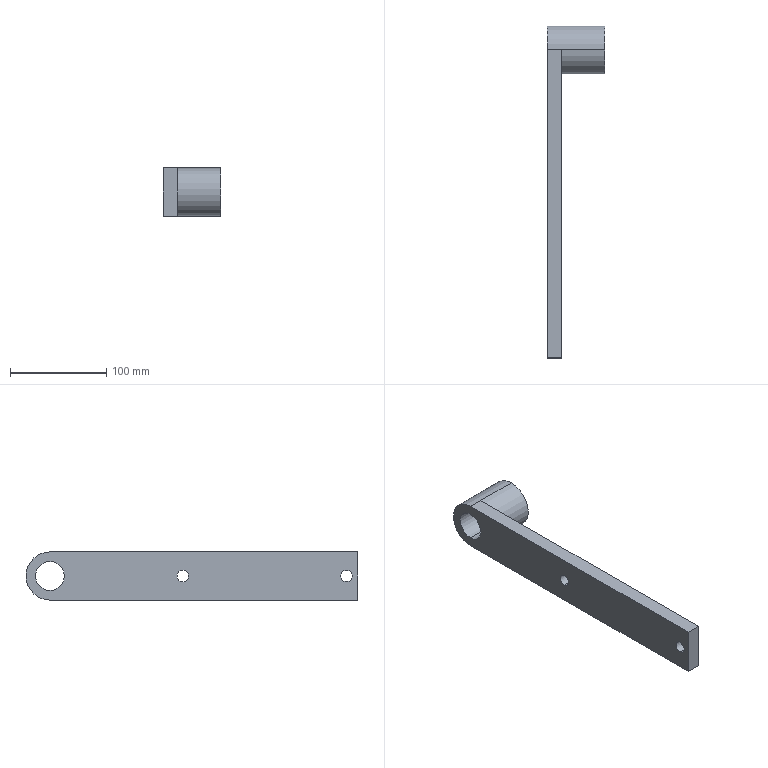Part | SolidWorks | features ICE 2, Extrusion 1, HoleWzd 1 | 1 solid | 14 faces | box 60 x 345 x 50 mm | volume 297279 mm3 | cylinder 8 | plane 6 | commonest cylinder face diameters 12 x4 30 x2 50 x2
STEP:
#1=CARTESIAN_POINT('',(7.5,22.,6.));
#2=VERTEX_POINT('',#1);
#3=CARTESIAN_POINT('',(7.5,22.,-6.));
#4=VERTEX_POINT('',#3);
#5=CARTESIAN_POINT('',(7.5,22.,0.));
#6=DIRECTION('',(1.,0.,0.));
#7=DIRECTION('',(0.,0.,-1.));
#8=AXIS2_PLACEMENT_3D('',#5,#6,#7);
#9=CIRCLE('',#8,6.);
#10=EDGE_CURVE('',#2,#4,#9,.T.);
#11=ORIENTED_EDGE('',*,*,#10,.T.);
#12=CARTESIAN_POINT('',(-7.5,22.,-6.));
#13=VERTEX_POINT('',#12);
#14=CARTESIAN_POINT('',(-7.5,22.,-6.));
#15=DIRECTION('',(-1.,0.,0.));
#16=VECTOR('',#15,1000.);
#17=LINE('',#14,#16);
#18=EDGE_CURVE('',#4,#13,#17,.T.);
#19=ORIENTED_EDGE('',*,*,#18,.T.);
#20=CARTESIAN_POINT('',(-7.5,22.,6.));
#21=VERTEX_POINT('',#20);
#22=CARTESIAN_POINT('',(-7.5,22.,0.));
#23=DIRECTION('',(-1.,0.,0.));
#24=DIRECTION('',(0.,0.,1.));
#25=AXIS2_PLACEMENT_3D('',#22,#23,#24);
#26=CIRCLE('',#25,6.);
#27=EDGE_CURVE('',#13,#21,#26,.T.);
#28=ORIENTED_EDGE('',*,*,#27,.T.);
#29=CARTESIAN_POINT('',(-7.5,22.,6.));
#30=DIRECTION('',(-1.,0.,0.));
#31=VECTOR('',#30,1000.);
#32=LINE('',#29,#31);
#33=EDGE_CURVE('',#2,#21,#32,.T.);
#34=ORIENTED_EDGE('',*,*,#33,.F.);
#35=EDGE_LOOP('',(#11,#19,#28,#34));
#36=FACE_OUTER_BOUND('',#35,.T.);
#37=CARTESIAN_POINT('',(-7.5,22.,0.));
#38=DIRECTION('',(-1.,0.,0.));
#39=DIRECTION('',(0.,0.,1.));
#40=AXIS2_PLACEMENT_3D('',#37,#38,#39);
#41=CYLINDRICAL_SURFACE('',#40,6.);
#42=ADVANCED_FACE('',(#36),#41,.F.);
#43=CARTESIAN_POINT('',(7.5,-148.,6.));
#44=VERTEX_POINT('',#43);
#45=CARTESIAN_POINT('',(7.5,-148.,-6.));
#46=VERTEX_POINT('',#45);
#47=CARTESIAN_POINT('',(7.5,-148.,0.));
#48=DIRECTION('',(1.,0.,0.));
#49=DIRECTION('',(0.,0.,-1.));
#50=AXIS2_PLACEMENT_3D('',#47,#48,#49);
#51=CIRCLE('',#50,6.);
#52=EDGE_CURVE('',#44,#46,#51,.T.);
#53=ORIENTED_EDGE('',*,*,#52,.T.);
#54=CARTESIAN_POINT('',(-7.5,-148.,-6.));
#55=VERTEX_POINT('',#54);
#56=CARTESIAN_POINT('',(-7.5,-148.,-6.));
#57=DIRECTION('',(-1.,0.,0.));
#58=VECTOR('',#57,1000.);
#59=LINE('',#56,#58);
#60=EDGE_CURVE('',#46,#55,#59,.T.);
#61=ORIENTED_EDGE('',*,*,#60,.T.);
#62=CARTESIAN_POINT('',(-7.5,-148.,6.));
#63=VERTEX_POINT('',#62);
#64=CARTESIAN_POINT('',(-7.5,-148.,0.));
#65=DIRECTION('',(-1.,0.,0.));
#66=DIRECTION('',(0.,0.,1.));
#67=AXIS2_PLACEMENT_3D('',#64,#65,#66);
#68=CIRCLE('',#67,6.);
#69=EDGE_CURVE('',#55,#63,#68,.T.);
#70=ORIENTED_EDGE('',*,*,#69,.T.);
#71=CARTESIAN_POINT('',(-7.5,-148.,6.));
#72=DIRECTION('',(-1.,0.,0.));
#73=VECTOR('',#72,1000.);
#74=LINE('',#71,#73);
#75=EDGE_CURVE('',#44,#63,#74,.T.);
#76=ORIENTED_EDGE('',*,*,#75,.F.);
#77=EDGE_LOOP('',(#53,#61,#70,#76));
#78=FACE_OUTER_BOUND('',#77,.T.);
#79=CARTESIAN_POINT('',(-7.5,-148.,0.));
#80=DIRECTION('',(-1.,0.,0.));
#81=DIRECTION('',(0.,0.,1.));
#82=AXIS2_PLACEMENT_3D('',#79,#80,#81);
#83=CYLINDRICAL_SURFACE('',#82,6.);
#84=ADVANCED_FACE('',(#78),#83,.F.);
#85=CARTESIAN_POINT('',(-7.5,160.,15.));
#86=VERTEX_POINT('',#85);
#87=CARTESIAN_POINT('',(-7.5,160.,-15.));
#88=VERTEX_POINT('',#87);
#89=CARTESIAN_POINT('',(-7.5,160.,0.));
#90=DIRECTION('',(1.,0.,0.));
#91=DIRECTION('',(0.,0.,-1.));
#92=AXIS2_PLACEMENT_3D('',#89,#90,#91);
#93=CIRCLE('',#92,15.);
#94=EDGE_CURVE('',#86,#88,#93,.T.);
#95=ORIENTED_EDGE('',*,*,#94,.F.);
#96=CARTESIAN_POINT('',(52.5,160.,15.));
#97=VERTEX_POINT('',#96);
#98=CARTESIAN_POINT('',(-7.5,160.,15.));
#99=DIRECTION('',(1.,0.,0.));
#100=VECTOR('',#99,1000.);
#101=LINE('',#98,#100);
#102=EDGE_CURVE('',#86,#97,#101,.T.);
#103=ORIENTED_EDGE('',*,*,#102,.T.);
#104=CARTESIAN_POINT('',(52.5,160.,-15.));
#105=VERTEX_POINT('',#104);
#106=CARTESIAN_POINT('',(52.5,160.,0.));
#107=DIRECTION('',(1.,0.,0.));
#108=DIRECTION('',(0.,0.,-1.));
#109=AXIS2_PLACEMENT_3D('',#106,#107,#108);
#110=CIRCLE('',#109,15.);
#111=EDGE_CURVE('',#97,#105,#110,.T.);
#112=ORIENTED_EDGE('',*,*,#111,.T.);
#113=CARTESIAN_POINT('',(-7.5,160.,-15.));
#114=DIRECTION('',(1.,0.,0.));
#115=VECTOR('',#114,1000.);
#116=LINE('',#113,#115);
#117=EDGE_CURVE('',#88,#105,#116,.T.);
#118=ORIENTED_EDGE('',*,*,#117,.F.);
#119=EDGE_LOOP('',(#95,#103,#112,#118));
#120=FACE_OUTER_BOUND('',#119,.T.);
#121=CARTESIAN_POINT('',(-7.5,160.,0.));
#122=DIRECTION('',(1.,0.,0.));
#123=DIRECTION('',(0.,0.,-1.));
#124=AXIS2_PLACEMENT_3D('',#121,#122,#123);
#125=CYLINDRICAL_SURFACE('',#124,15.);
#126=ADVANCED_FACE('',(#120),#125,.F.);
#127=CARTESIAN_POINT('',(7.5,160.,25.));
#128=VERTEX_POINT('',#127);
#129=CARTESIAN_POINT('',(-7.5,160.,25.));
#130=VERTEX_POINT('',#129);
#131=CARTESIAN_POINT('',(7.5,160.,25.));
#132=DIRECTION('',(-1.,0.,0.));
#133=VECTOR('',#132,1000.);
#134=LINE('',#131,#133);
#135=EDGE_CURVE('',#128,#130,#134,.T.);
#136=ORIENTED_EDGE('',*,*,#135,.F.);
#137=CARTESIAN_POINT('',(52.5,160.,25.));
#138=VERTEX_POINT('',#137);
#139=CARTESIAN_POINT('',(-7.5,160.,25.));
#140=DIRECTION('',(1.,0.,0.));
#141=VECTOR('',#140,1000.);
#142=LINE('',#139,#141);
#143=EDGE_CURVE('',#128,#138,#142,.T.);
#144=ORIENTED_EDGE('',*,*,#143,.T.);
#145=CARTESIAN_POINT('',(52.5,160.,-25.));
#146=VERTEX_POINT('',#145);
#147=CARTESIAN_POINT('',(52.5,160.,0.));
#148=DIRECTION('',(1.,0.,0.));
#149=DIRECTION('',(0.,0.,-1.));
#150=AXIS2_PLACEMENT_3D('',#147,#148,#149);
#151=CIRCLE('',#150,25.);
#152=EDGE_CURVE('',#146,#138,#151,.T.);
#153=ORIENTED_EDGE('',*,*,#152,.F.);
#154=CARTESIAN_POINT('',(7.5,160.,-25.));
#155=VERTEX_POINT('',#154);
#156=CARTESIAN_POINT('',(-7.5,160.,-25.));
#157=DIRECTION('',(1.,0.,0.));
#158=VECTOR('',#157,1000.);
#159=LINE('',#156,#158);
#160=EDGE_CURVE('',#155,#146,#159,.T.);
#161=ORIENTED_EDGE('',*,*,#160,.F.);
#162=CARTESIAN_POINT('',(-7.5,160.,-25.));
#163=VERTEX_POINT('',#162);
#164=CARTESIAN_POINT('',(7.5,160.,-25.));
#165=DIRECTION('',(-1.,0.,0.));
#166=VECTOR('',#165,1000.);
#167=LINE('',#164,#166);
#168=EDGE_CURVE('',#155,#163,#167,.T.);
#169=ORIENTED_EDGE('',*,*,#168,.T.);
#170=CARTESIAN_POINT('',(-7.5,160.,0.));
#171=DIRECTION('',(1.,0.,0.));
#172=DIRECTION('',(0.,0.,-1.));
#173=AXIS2_PLACEMENT_3D('',#170,#171,#172);
#174=CIRCLE('',#173,25.);
#175=EDGE_CURVE('',#163,#130,#174,.T.);
#176=ORIENTED_EDGE('',*,*,#175,.T.);
#177=EDGE_LOOP('',(#136,#144,#153,#161,#169,#176));
#178=FACE_OUTER_BOUND('',#177,.T.);
#179=CARTESIAN_POINT('',(-7.5,160.,0.));
#180=DIRECTION('',(1.,0.,0.));
#181=DIRECTION('',(0.,0.,-1.));
#182=AXIS2_PLACEMENT_3D('',#179,#180,#181);
#183=CYLINDRICAL_SURFACE('',#182,25.);
#184=ADVANCED_FACE('',(#178),#183,.T.);
#185=CARTESIAN_POINT('',(-7.5,-160.,-25.));
#186=VERTEX_POINT('',#185);
#187=CARTESIAN_POINT('',(-7.5,160.,-25.));
#188=DIRECTION('',(0.,1.,0.));
#189=VECTOR('',#188,1000.);
#190=LINE('',#187,#189);
#191=EDGE_CURVE('',#186,#163,#190,.T.);
#192=ORIENTED_EDGE('',*,*,#191,.T.);
#193=ORIENTED_EDGE('',*,*,#168,.F.);
#194=CARTESIAN_POINT('',(7.5,-160.,-25.));
#195=VERTEX_POINT('',#194);
#196=CARTESIAN_POINT('',(7.5,160.,-25.));
#197=DIRECTION('',(0.,1.,0.));
#198=VECTOR('',#197,1000.);
#199=LINE('',#196,#198);
#200=EDGE_CURVE('',#195,#155,#199,.T.);
#201=ORIENTED_EDGE('',*,*,#200,.F.);
#202=CARTESIAN_POINT('',(7.5,-160.,-25.));
#203=DIRECTION('',(-1.,0.,0.));
#204=VECTOR('',#203,1000.);
#205=LINE('',#202,#204);
#206=EDGE_CURVE('',#195,#186,#205,.T.);
#207=ORIENTED_EDGE('',*,*,#206,.T.);
#208=EDGE_LOOP('',(#192,#193,#201,#207));
#209=FACE_OUTER_BOUND('',#208,.T.);
#210=CARTESIAN_POINT('',(7.5,160.,-25.));
#211=DIRECTION('',(0.,0.,1.));
#212=DIRECTION('',(0.,-1.,0.));
#213=AXIS2_PLACEMENT_3D('',#210,#211,#212);
#214=PLANE('',#213);
#215=ADVANCED_FACE('',(#209),#214,.F.);
#216=CARTESIAN_POINT('',(-7.5,-160.,25.));
#217=VERTEX_POINT('',#216);
#218=CARTESIAN_POINT('',(-7.5,160.,25.));
#219=DIRECTION('',(0.,-1.,0.));
#220=VECTOR('',#219,1000.);
#221=LINE('',#218,#220);
#222=EDGE_CURVE('',#130,#217,#221,.T.);
#223=ORIENTED_EDGE('',*,*,#222,.T.);
#224=CARTESIAN_POINT('',(7.5,-160.,25.));
#225=VERTEX_POINT('',#224);
#226=CARTESIAN_POINT('',(7.5,-160.,25.));
#227=DIRECTION('',(-1.,0.,0.));
#228=VECTOR('',#227,1000.);
#229=LINE('',#226,#228);
#230=EDGE_CURVE('',#225,#217,#229,.T.);
#231=ORIENTED_EDGE('',*,*,#230,.F.);
#232=CARTESIAN_POINT('',(7.5,160.,25.));
#233=DIRECTION('',(0.,-1.,0.));
#234=VECTOR('',#233,1000.);
#235=LINE('',#232,#234);
#236=EDGE_CURVE('',#128,#225,#235,.T.);
#237=ORIENTED_EDGE('',*,*,#236,.F.);
#238=ORIENTED_EDGE('',*,*,#135,.T.);
#239=EDGE_LOOP('',(#223,#231,#237,#238));
#240=FACE_OUTER_BOUND('',#239,.T.);
#241=CARTESIAN_POINT('',(7.5,160.,25.));
#242=DIRECTION('',(0.,0.,-1.));
#243=DIRECTION('',(0.,1.,0.));
#244=AXIS2_PLACEMENT_3D('',#241,#242,#243);
#245=PLANE('',#244);
#246=ADVANCED_FACE('',(#240),#245,.F.);
#247=CARTESIAN_POINT('',(-7.5,-160.,25.));
#248=DIRECTION('',(0.,0.,-1.));
#249=VECTOR('',#248,1000.);
#250=LINE('',#247,#249);
#251=EDGE_CURVE('',#217,#186,#250,.T.);
#252=ORIENTED_EDGE('',*,*,#251,.T.);
#253=ORIENTED_EDGE('',*,*,#206,.F.);
#254=CARTESIAN_POINT('',(7.5,-160.,25.));
#255=DIRECTION('',(0.,0.,-1.));
#256=VECTOR('',#255,1000.);
#257=LINE('',#254,#256);
#258=EDGE_CURVE('',#225,#195,#257,.T.);
#259=ORIENTED_EDGE('',*,*,#258,.F.);
#260=ORIENTED_EDGE('',*,*,#230,.T.);
#261=EDGE_LOOP('',(#252,#253,#259,#260));
#262=FACE_OUTER_BOUND('',#261,.T.);
#263=CARTESIAN_POINT('',(7.5,-160.,25.));
#264=DIRECTION('',(0.,1.,0.));
#265=DIRECTION('',(0.,0.,1.));
#266=AXIS2_PLACEMENT_3D('',#263,#264,#265);
#267=PLANE('',#266);
#268=ADVANCED_FACE('',(#262),#267,.F.);
#269=ORIENTED_EDGE('',*,*,#10,.F.);
#270=CARTESIAN_POINT('',(7.5,22.,0.));
#271=DIRECTION('',(1.,0.,0.));
#272=DIRECTION('',(0.,0.,-1.));
#273=AXIS2_PLACEMENT_3D('',#270,#271,#272);
#274=CIRCLE('',#273,6.);
#275=EDGE_CURVE('',#4,#2,#274,.T.);
#276=ORIENTED_EDGE('',*,*,#275,.F.);
#277=EDGE_LOOP('',(#269,#276));
#278=FACE_BOUND('',#277,.T.);
#279=ORIENTED_EDGE('',*,*,#52,.F.);
#280=CARTESIAN_POINT('',(7.5,-148.,0.));
#281=DIRECTION('',(1.,0.,0.));
#282=DIRECTION('',(0.,0.,-1.));
#283=AXIS2_PLACEMENT_3D('',#280,#281,#282);
#284=CIRCLE('',#283,6.);
#285=EDGE_CURVE('',#46,#44,#284,.T.);
#286=ORIENTED_EDGE('',*,*,#285,.F.);
#287=EDGE_LOOP('',(#279,#286));
#288=FACE_BOUND('',#287,.T.);
#289=CARTESIAN_POINT('',(7.5,160.,0.));
#290=DIRECTION('',(1.,0.,0.));
#291=DIRECTION('',(0.,0.,-1.));
#292=AXIS2_PLACEMENT_3D('',#289,#290,#291);
#293=CIRCLE('',#292,25.);
#294=EDGE_CURVE('',#128,#155,#293,.T.);
#295=ORIENTED_EDGE('',*,*,#294,.F.);
#296=ORIENTED_EDGE('',*,*,#236,.T.);
#297=ORIENTED_EDGE('',*,*,#258,.T.);
#298=ORIENTED_EDGE('',*,*,#200,.T.);
#299=EDGE_LOOP('',(#295,#296,#297,#298));
#300=FACE_OUTER_BOUND('',#299,.T.);
#301=CARTESIAN_POINT('',(7.5,0.,0.));
#302=DIRECTION('',(1.,0.,0.));
#303=DIRECTION('',(0.,0.,-1.));
#304=AXIS2_PLACEMENT_3D('',#301,#302,#303);
#305=PLANE('',#304);
#306=ADVANCED_FACE('',(#278,#288,#300),#305,.T.);
#307=CARTESIAN_POINT('',(-7.5,22.,0.));
#308=DIRECTION('',(-1.,0.,0.));
#309=DIRECTION('',(0.,0.,1.));
#310=AXIS2_PLACEMENT_3D('',#307,#308,#309);
#311=CIRCLE('',#310,6.);
#312=EDGE_CURVE('',#21,#13,#311,.T.);
#313=ORIENTED_EDGE('',*,*,#312,.F.);
#314=ORIENTED_EDGE('',*,*,#27,.F.);
#315=EDGE_LOOP('',(#313,#314));
#316=FACE_BOUND('',#315,.T.);
#317=CARTESIAN_POINT('',(-7.5,-148.,0.));
#318=DIRECTION('',(-1.,0.,0.));
#319=DIRECTION('',(0.,0.,1.));
#320=AXIS2_PLACEMENT_3D('',#317,#318,#319);
#321=CIRCLE('',#320,6.);
#322=EDGE_CURVE('',#63,#55,#321,.T.);
#323=ORIENTED_EDGE('',*,*,#322,.F.);
#324=ORIENTED_EDGE('',*,*,#69,.F.);
#325=EDGE_LOOP('',(#323,#324));
#326=FACE_BOUND('',#325,.T.);
#327=CARTESIAN_POINT('',(-7.5,160.,0.));
#328=DIRECTION('',(1.,0.,0.));
#329=DIRECTION('',(0.,0.,-1.));
#330=AXIS2_PLACEMENT_3D('',#327,#328,#329);
#331=CIRCLE('',#330,15.);
#332=EDGE_CURVE('',#88,#86,#331,.T.);
#333=ORIENTED_EDGE('',*,*,#332,.T.);
#334=ORIENTED_EDGE('',*,*,#94,.T.);
#335=EDGE_LOOP('',(#333,#334));
#336=FACE_BOUND('',#335,.T.);
#337=ORIENTED_EDGE('',*,*,#222,.F.);
#338=ORIENTED_EDGE('',*,*,#175,.F.);
#339=ORIENTED_EDGE('',*,*,#191,.F.);
#340=ORIENTED_EDGE('',*,*,#251,.F.);
#341=EDGE_LOOP('',(#337,#338,#339,#340));
#342=FACE_OUTER_BOUND('',#341,.T.);
#343=CARTESIAN_POINT('',(-7.5,0.,0.));
#344=DIRECTION('',(1.,0.,0.));
#345=DIRECTION('',(0.,0.,-1.));
#346=AXIS2_PLACEMENT_3D('',#343,#344,#345);
#347=PLANE('',#346);
#348=ADVANCED_FACE('',(#316,#326,#336,#342),#347,.F.);
#349=ORIENTED_EDGE('',*,*,#143,.F.);
#350=ORIENTED_EDGE('',*,*,#294,.T.);
#351=ORIENTED_EDGE('',*,*,#160,.T.);
#352=CARTESIAN_POINT('',(52.5,160.,0.));
#353=DIRECTION('',(1.,0.,0.));
#354=DIRECTION('',(0.,0.,-1.));
#355=AXIS2_PLACEMENT_3D('',#352,#353,#354);
#356=CIRCLE('',#355,25.);
#357=EDGE_CURVE('',#138,#146,#356,.T.);
#358=ORIENTED_EDGE('',*,*,#357,.F.);
#359=EDGE_LOOP('',(#349,#350,#351,#358));
#360=FACE_OUTER_BOUND('',#359,.T.);
#361=CARTESIAN_POINT('',(-7.5,160.,0.));
#362=DIRECTION('',(1.,0.,0.));
#363=DIRECTION('',(0.,0.,-1.));
#364=AXIS2_PLACEMENT_3D('',#361,#362,#363);
#365=CYLINDRICAL_SURFACE('',#364,25.);
#366=ADVANCED_FACE('',(#360),#365,.T.);
#367=CARTESIAN_POINT('',(52.5,160.,0.));
#368=DIRECTION('',(1.,0.,0.));
#369=DIRECTION('',(0.,0.,-1.));
#370=AXIS2_PLACEMENT_3D('',#367,#368,#369);
#371=CIRCLE('',#370,15.);
#372=EDGE_CURVE('',#105,#97,#371,.T.);
#373=ORIENTED_EDGE('',*,*,#372,.F.);
#374=ORIENTED_EDGE('',*,*,#111,.F.);
#375=EDGE_LOOP('',(#373,#374));
#376=FACE_BOUND('',#375,.T.);
#377=ORIENTED_EDGE('',*,*,#152,.T.);
#378=ORIENTED_EDGE('',*,*,#357,.T.);
#379=EDGE_LOOP('',(#377,#378));
#380=FACE_OUTER_BOUND('',#379,.T.);
#381=CARTESIAN_POINT('',(52.5,160.,0.));
#382=DIRECTION('',(1.,0.,0.));
#383=DIRECTION('',(0.,0.,-1.));
#384=AXIS2_PLACEMENT_3D('',#381,#382,#383);
#385=PLANE('',#384);
#386=ADVANCED_FACE('',(#376,#380),#385,.T.);
#387=ORIENTED_EDGE('',*,*,#102,.F.);
#388=ORIENTED_EDGE('',*,*,#332,.F.);
#389=ORIENTED_EDGE('',*,*,#117,.T.);
#390=ORIENTED_EDGE('',*,*,#372,.T.);
#391=EDGE_LOOP('',(#387,#388,#389,#390));
#392=FACE_OUTER_BOUND('',#391,.T.);
#393=CARTESIAN_POINT('',(-7.5,160.,0.));
#394=DIRECTION('',(1.,0.,0.));
#395=DIRECTION('',(0.,0.,-1.));
#396=AXIS2_PLACEMENT_3D('',#393,#394,#395);
#397=CYLINDRICAL_SURFACE('',#396,15.);
#398=ADVANCED_FACE('',(#392),#397,.F.);
#399=ORIENTED_EDGE('',*,*,#60,.F.);
#400=ORIENTED_EDGE('',*,*,#285,.T.);
#401=ORIENTED_EDGE('',*,*,#75,.T.);
#402=ORIENTED_EDGE('',*,*,#322,.T.);
#403=EDGE_LOOP('',(#399,#400,#401,#402));
#404=FACE_OUTER_BOUND('',#403,.T.);
#405=CARTESIAN_POINT('',(-7.5,-148.,0.));
#406=DIRECTION('',(-1.,0.,0.));
#407=DIRECTION('',(0.,0.,1.));
#408=AXIS2_PLACEMENT_3D('',#405,#406,#407);
#409=CYLINDRICAL_SURFACE('',#408,6.);
#410=ADVANCED_FACE('',(#404),#409,.F.);
#411=ORIENTED_EDGE('',*,*,#18,.F.);
#412=ORIENTED_EDGE('',*,*,#275,.T.);
#413=ORIENTED_EDGE('',*,*,#33,.T.);
#414=ORIENTED_EDGE('',*,*,#312,.T.);
#415=EDGE_LOOP('',(#411,#412,#413,#414));
#416=FACE_OUTER_BOUND('',#415,.T.);
#417=CARTESIAN_POINT('',(-7.5,22.,0.));
#418=DIRECTION('',(-1.,0.,0.));
#419=DIRECTION('',(0.,0.,1.));
#420=AXIS2_PLACEMENT_3D('',#417,#418,#419);
#421=CYLINDRICAL_SURFACE('',#420,6.);
#422=ADVANCED_FACE('',(#416),#421,.F.);
#423=CLOSED_SHELL('',(#42,#84,#126,#184,#215,#246,#268,#306,#348,#366,#386,#398,#410,#422));
#424=MANIFOLD_SOLID_BREP('',#423);
#425=CARTESIAN_POINT('',(0.,0.,0.));
#426=DIRECTION('',(0.,0.,1.));
#427=DIRECTION('',(1.,0.,0.));
#428=AXIS2_PLACEMENT_3D('',#425,#426,#427);
#429=(LENGTH_UNIT()NAMED_UNIT(*)SI_UNIT(.MILLI.,.METRE.));
#430=UNCERTAINTY_MEASURE_WITH_UNIT(LENGTH_MEASURE(0.00001),#429,'','');
#431=(NAMED_UNIT(*)PLANE_ANGLE_UNIT()SI_UNIT($,.RADIAN.));
#432=(NAMED_UNIT(*)SI_UNIT($,.STERADIAN.)SOLID_ANGLE_UNIT());
#433=(GEOMETRIC_REPRESENTATION_CONTEXT(3)GLOBAL_UNCERTAINTY_ASSIGNED_CONTEXT((#430))GLOBAL_UNIT_ASSIGNED_CONTEXT((#429,#431,#432))REPRESENTATION_CONTEXT('',''));
#434=ADVANCED_BREP_SHAPE_REPRESENTATION('',(#424,#428),#433);